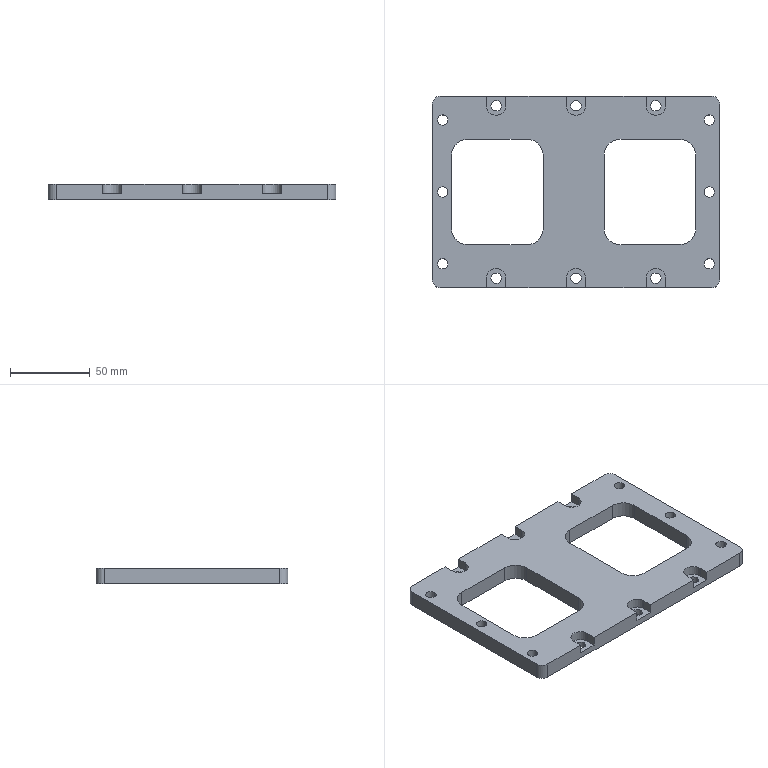Part | STEP file | 03-16 trimming support bracket | 1 solid | 74 faces | box 180 x 120 x 10 mm | volume 134253 mm3 | cylinder 42 | plane 32 | commonest cylinder face diameters 6.5 x24 20 x8 12 x6 10 x4